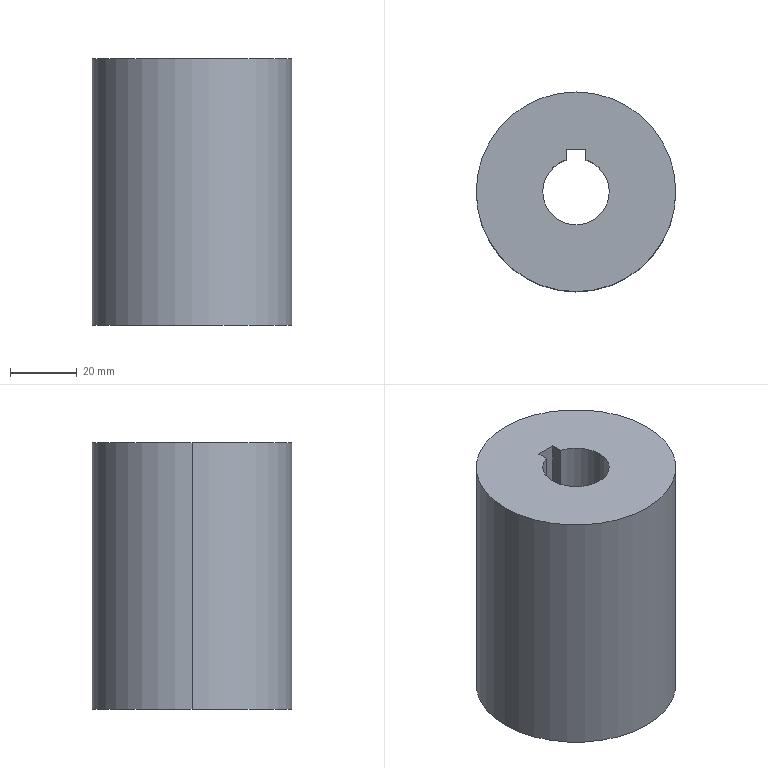Part | SolidWorks | features ICE 4, Extrusion 1 | 1 solid | 15 faces | box 60 x 60 x 80 mm | volume 183532 mm3 | plane 9 | cylinder 6 | commonest cylinder face diameters 20 x3 60 x2 30 x1
STEP:
#1=CARTESIAN_POINT('',(30.,0.,40.));
#2=VERTEX_POINT('',#1);
#3=CARTESIAN_POINT('',(-30.,0.,40.));
#4=VERTEX_POINT('',#3);
#5=CARTESIAN_POINT('',(0.,0.,40.));
#6=DIRECTION('',(0.,0.,1.));
#7=DIRECTION('',(1.,0.,0.));
#8=AXIS2_PLACEMENT_3D('',#5,#6,#7);
#9=CIRCLE('',#8,30.);
#10=EDGE_CURVE('',#2,#4,#9,.T.);
#11=ORIENTED_EDGE('',*,*,#10,.F.);
#12=CARTESIAN_POINT('',(30.,0.,-40.));
#13=VERTEX_POINT('',#12);
#14=CARTESIAN_POINT('',(30.,0.,40.));
#15=DIRECTION('',(0.,0.,-1.));
#16=VECTOR('',#15,1000.);
#17=LINE('',#14,#16);
#18=EDGE_CURVE('',#2,#13,#17,.T.);
#19=ORIENTED_EDGE('',*,*,#18,.T.);
#20=CARTESIAN_POINT('',(-30.,0.,-40.));
#21=VERTEX_POINT('',#20);
#22=CARTESIAN_POINT('',(0.,0.,-40.));
#23=DIRECTION('',(0.,0.,1.));
#24=DIRECTION('',(1.,0.,0.));
#25=AXIS2_PLACEMENT_3D('',#22,#23,#24);
#26=CIRCLE('',#25,30.);
#27=EDGE_CURVE('',#13,#21,#26,.T.);
#28=ORIENTED_EDGE('',*,*,#27,.T.);
#29=CARTESIAN_POINT('',(-30.,0.,40.));
#30=DIRECTION('',(0.,0.,-1.));
#31=VECTOR('',#30,1000.);
#32=LINE('',#29,#31);
#33=EDGE_CURVE('',#4,#21,#32,.T.);
#34=ORIENTED_EDGE('',*,*,#33,.F.);
#35=EDGE_LOOP('',(#11,#19,#28,#34));
#36=FACE_OUTER_BOUND('',#35,.T.);
#37=CARTESIAN_POINT('',(0.,0.,40.));
#38=DIRECTION('',(0.,0.,-1.));
#39=DIRECTION('',(-1.,0.,0.));
#40=AXIS2_PLACEMENT_3D('',#37,#38,#39);
#41=CYLINDRICAL_SURFACE('',#40,30.);
#42=ADVANCED_FACE('',(#36),#41,.T.);
#43=CARTESIAN_POINT('',(-10.,0.,0.));
#44=VERTEX_POINT('',#43);
#45=CARTESIAN_POINT('',(10.,0.,0.));
#46=VERTEX_POINT('',#45);
#47=CARTESIAN_POINT('',(0.,0.,0.));
#48=DIRECTION('',(0.,0.,1.));
#49=DIRECTION('',(-1.,0.,0.));
#50=AXIS2_PLACEMENT_3D('',#47,#48,#49);
#51=CIRCLE('',#50,10.);
#52=EDGE_CURVE('',#44,#46,#51,.T.);
#53=ORIENTED_EDGE('',*,*,#52,.F.);
#54=CARTESIAN_POINT('',(-10.,0.,40.));
#55=VERTEX_POINT('',#54);
#56=CARTESIAN_POINT('',(-10.,0.,-40.));
#57=DIRECTION('',(0.,0.,1.));
#58=VECTOR('',#57,1000.);
#59=LINE('',#56,#58);
#60=EDGE_CURVE('',#44,#55,#59,.T.);
#61=ORIENTED_EDGE('',*,*,#60,.T.);
#62=CARTESIAN_POINT('',(10.,0.,40.));
#63=VERTEX_POINT('',#62);
#64=CARTESIAN_POINT('',(0.,0.,40.));
#65=DIRECTION('',(0.,0.,1.));
#66=DIRECTION('',(1.,0.,0.));
#67=AXIS2_PLACEMENT_3D('',#64,#65,#66);
#68=CIRCLE('',#67,10.);
#69=EDGE_CURVE('',#55,#63,#68,.T.);
#70=ORIENTED_EDGE('',*,*,#69,.T.);
#71=CARTESIAN_POINT('',(10.,0.,-40.));
#72=DIRECTION('',(0.,0.,1.));
#73=VECTOR('',#72,1000.);
#74=LINE('',#71,#73);
#75=EDGE_CURVE('',#46,#63,#74,.T.);
#76=ORIENTED_EDGE('',*,*,#75,.F.);
#77=EDGE_LOOP('',(#53,#61,#70,#76));
#78=FACE_OUTER_BOUND('',#77,.T.);
#79=CARTESIAN_POINT('',(0.,0.,-40.));
#80=DIRECTION('',(0.,0.,1.));
#81=DIRECTION('',(1.,0.,0.));
#82=AXIS2_PLACEMENT_3D('',#79,#80,#81);
#83=CYLINDRICAL_SURFACE('',#82,10.);
#84=ADVANCED_FACE('',(#78),#83,.F.);
#85=CARTESIAN_POINT('',(3.,9.539,0.));
#86=VERTEX_POINT('',#85);
#87=CARTESIAN_POINT('',(0.,0.,0.));
#88=DIRECTION('',(0.,0.,1.));
#89=DIRECTION('',(-1.,0.,0.));
#90=AXIS2_PLACEMENT_3D('',#87,#88,#89);
#91=CIRCLE('',#90,10.);
#92=EDGE_CURVE('',#46,#86,#91,.T.);
#93=ORIENTED_EDGE('',*,*,#92,.F.);
#94=ORIENTED_EDGE('',*,*,#75,.T.);
#95=CARTESIAN_POINT('',(3.,9.539,40.));
#96=VERTEX_POINT('',#95);
#97=CARTESIAN_POINT('',(0.,0.,40.));
#98=DIRECTION('',(0.,0.,1.));
#99=DIRECTION('',(1.,0.,0.));
#100=AXIS2_PLACEMENT_3D('',#97,#98,#99);
#101=CIRCLE('',#100,10.);
#102=EDGE_CURVE('',#63,#96,#101,.T.);
#103=ORIENTED_EDGE('',*,*,#102,.T.);
#104=CARTESIAN_POINT('',(3.,9.539,-40.));
#105=DIRECTION('',(0.,0.,-1.));
#106=VECTOR('',#105,1000.);
#107=LINE('',#104,#106);
#108=EDGE_CURVE('',#96,#86,#107,.T.);
#109=ORIENTED_EDGE('',*,*,#108,.T.);
#110=EDGE_LOOP('',(#93,#94,#103,#109));
#111=FACE_OUTER_BOUND('',#110,.T.);
#112=CARTESIAN_POINT('',(0.,0.,-40.));
#113=DIRECTION('',(0.,0.,1.));
#114=DIRECTION('',(1.,0.,0.));
#115=AXIS2_PLACEMENT_3D('',#112,#113,#114);
#116=CYLINDRICAL_SURFACE('',#115,10.);
#117=ADVANCED_FACE('',(#111),#116,.F.);
#118=ORIENTED_EDGE('',*,*,#60,.F.);
#119=CARTESIAN_POINT('',(-3.,9.539,0.));
#120=VERTEX_POINT('',#119);
#121=CARTESIAN_POINT('',(0.,0.,0.));
#122=DIRECTION('',(0.,0.,1.));
#123=DIRECTION('',(-1.,0.,0.));
#124=AXIS2_PLACEMENT_3D('',#121,#122,#123);
#125=CIRCLE('',#124,10.);
#126=EDGE_CURVE('',#120,#44,#125,.T.);
#127=ORIENTED_EDGE('',*,*,#126,.F.);
#128=CARTESIAN_POINT('',(-3.,9.539,40.));
#129=VERTEX_POINT('',#128);
#130=CARTESIAN_POINT('',(-3.,9.539,-40.));
#131=DIRECTION('',(0.,0.,1.));
#132=VECTOR('',#131,1000.);
#133=LINE('',#130,#132);
#134=EDGE_CURVE('',#120,#129,#133,.T.);
#135=ORIENTED_EDGE('',*,*,#134,.T.);
#136=CARTESIAN_POINT('',(0.,0.,40.));
#137=DIRECTION('',(0.,0.,1.));
#138=DIRECTION('',(1.,0.,0.));
#139=AXIS2_PLACEMENT_3D('',#136,#137,#138);
#140=CIRCLE('',#139,10.);
#141=EDGE_CURVE('',#129,#55,#140,.T.);
#142=ORIENTED_EDGE('',*,*,#141,.T.);
#143=EDGE_LOOP('',(#118,#127,#135,#142));
#144=FACE_OUTER_BOUND('',#143,.T.);
#145=CARTESIAN_POINT('',(0.,0.,-40.));
#146=DIRECTION('',(0.,0.,1.));
#147=DIRECTION('',(1.,0.,0.));
#148=AXIS2_PLACEMENT_3D('',#145,#146,#147);
#149=CYLINDRICAL_SURFACE('',#148,10.);
#150=ADVANCED_FACE('',(#144),#149,.F.);
#151=ORIENTED_EDGE('',*,*,#18,.F.);
#152=CARTESIAN_POINT('',(0.,0.,40.));
#153=DIRECTION('',(0.,0.,1.));
#154=DIRECTION('',(1.,0.,0.));
#155=AXIS2_PLACEMENT_3D('',#152,#153,#154);
#156=CIRCLE('',#155,30.);
#157=EDGE_CURVE('',#4,#2,#156,.T.);
#158=ORIENTED_EDGE('',*,*,#157,.F.);
#159=ORIENTED_EDGE('',*,*,#33,.T.);
#160=CARTESIAN_POINT('',(0.,0.,-40.));
#161=DIRECTION('',(0.,0.,1.));
#162=DIRECTION('',(1.,0.,0.));
#163=AXIS2_PLACEMENT_3D('',#160,#161,#162);
#164=CIRCLE('',#163,30.);
#165=EDGE_CURVE('',#21,#13,#164,.T.);
#166=ORIENTED_EDGE('',*,*,#165,.T.);
#167=EDGE_LOOP('',(#151,#158,#159,#166));
#168=FACE_OUTER_BOUND('',#167,.T.);
#169=CARTESIAN_POINT('',(0.,0.,40.));
#170=DIRECTION('',(0.,0.,-1.));
#171=DIRECTION('',(-1.,0.,0.));
#172=AXIS2_PLACEMENT_3D('',#169,#170,#171);
#173=CYLINDRICAL_SURFACE('',#172,30.);
#174=ADVANCED_FACE('',(#168),#173,.T.);
#175=CARTESIAN_POINT('',(-3.,12.8,40.));
#176=VERTEX_POINT('',#175);
#177=CARTESIAN_POINT('',(-3.,6.87,40.));
#178=DIRECTION('',(0.,-1.,0.));
#179=VECTOR('',#178,1000.);
#180=LINE('',#177,#179);
#181=EDGE_CURVE('',#176,#129,#180,.T.);
#182=ORIENTED_EDGE('',*,*,#181,.F.);
#183=CARTESIAN_POINT('',(3.,12.8,40.));
#184=VERTEX_POINT('',#183);
#185=CARTESIAN_POINT('',(3.,12.8,40.));
#186=DIRECTION('',(-1.,0.,0.));
#187=VECTOR('',#186,1000.);
#188=LINE('',#185,#187);
#189=EDGE_CURVE('',#184,#176,#188,.T.);
#190=ORIENTED_EDGE('',*,*,#189,.F.);
#191=CARTESIAN_POINT('',(3.,6.87,40.));
#192=DIRECTION('',(0.,1.,0.));
#193=VECTOR('',#192,1000.);
#194=LINE('',#191,#193);
#195=EDGE_CURVE('',#96,#184,#194,.T.);
#196=ORIENTED_EDGE('',*,*,#195,.F.);
#197=ORIENTED_EDGE('',*,*,#102,.F.);
#198=ORIENTED_EDGE('',*,*,#69,.F.);
#199=ORIENTED_EDGE('',*,*,#141,.F.);
#200=EDGE_LOOP('',(#182,#190,#196,#197,#198,#199));
#201=FACE_BOUND('',#200,.T.);
#202=ORIENTED_EDGE('',*,*,#157,.T.);
#203=ORIENTED_EDGE('',*,*,#10,.T.);
#204=EDGE_LOOP('',(#202,#203));
#205=FACE_OUTER_BOUND('',#204,.T.);
#206=CARTESIAN_POINT('',(0.,0.,40.));
#207=DIRECTION('',(0.,0.,1.));
#208=DIRECTION('',(1.,0.,0.));
#209=AXIS2_PLACEMENT_3D('',#206,#207,#208);
#210=PLANE('',#209);
#211=ADVANCED_FACE('',(#201,#205),#210,.T.);
#212=CARTESIAN_POINT('',(-14.457,4.,-40.));
#213=VERTEX_POINT('',#212);
#214=CARTESIAN_POINT('',(-14.457,-4.,-40.));
#215=VERTEX_POINT('',#214);
#216=CARTESIAN_POINT('',(0.,0.,-40.));
#217=DIRECTION('',(0.,0.,-1.));
#218=DIRECTION('',(-1.,0.,0.));
#219=AXIS2_PLACEMENT_3D('',#216,#217,#218);
#220=CIRCLE('',#219,15.);
#221=EDGE_CURVE('',#213,#215,#220,.T.);
#222=ORIENTED_EDGE('',*,*,#221,.F.);
#223=CARTESIAN_POINT('',(-18.3,4.,-40.));
#224=VERTEX_POINT('',#223);
#225=CARTESIAN_POINT('',(-18.3,4.,-40.));
#226=DIRECTION('',(1.,0.,0.));
#227=VECTOR('',#226,1000.);
#228=LINE('',#225,#227);
#229=EDGE_CURVE('',#224,#213,#228,.T.);
#230=ORIENTED_EDGE('',*,*,#229,.F.);
#231=CARTESIAN_POINT('',(-18.3,-4.,-40.));
#232=VERTEX_POINT('',#231);
#233=CARTESIAN_POINT('',(-18.3,-4.,-40.));
#234=DIRECTION('',(0.,1.,0.));
#235=VECTOR('',#234,1000.);
#236=LINE('',#233,#235);
#237=EDGE_CURVE('',#232,#224,#236,.T.);
#238=ORIENTED_EDGE('',*,*,#237,.F.);
#239=CARTESIAN_POINT('',(-18.3,-4.,-40.));
#240=DIRECTION('',(-1.,0.,0.));
#241=VECTOR('',#240,1000.);
#242=LINE('',#239,#241);
#243=EDGE_CURVE('',#215,#232,#242,.T.);
#244=ORIENTED_EDGE('',*,*,#243,.F.);
#245=EDGE_LOOP('',(#222,#230,#238,#244));
#246=FACE_BOUND('',#245,.T.);
#247=ORIENTED_EDGE('',*,*,#165,.F.);
#248=ORIENTED_EDGE('',*,*,#27,.F.);
#249=EDGE_LOOP('',(#247,#248));
#250=FACE_OUTER_BOUND('',#249,.T.);
#251=CARTESIAN_POINT('',(0.,0.,-40.));
#252=DIRECTION('',(0.,0.,1.));
#253=DIRECTION('',(1.,0.,0.));
#254=AXIS2_PLACEMENT_3D('',#251,#252,#253);
#255=PLANE('',#254);
#256=ADVANCED_FACE('',(#246,#250),#255,.F.);
#257=CARTESIAN_POINT('',(-18.3,4.,0.));
#258=VERTEX_POINT('',#257);
#259=CARTESIAN_POINT('',(-14.457,4.,0.));
#260=VERTEX_POINT('',#259);
#261=CARTESIAN_POINT('',(-18.3,4.,0.));
#262=DIRECTION('',(1.,0.,0.));
#263=VECTOR('',#262,1000.);
#264=LINE('',#261,#263);
#265=EDGE_CURVE('',#258,#260,#264,.T.);
#266=ORIENTED_EDGE('',*,*,#265,.T.);
#267=CARTESIAN_POINT('',(-14.457,-4.,0.));
#268=VERTEX_POINT('',#267);
#269=CARTESIAN_POINT('',(0.,0.,0.));
#270=DIRECTION('',(0.,0.,-1.));
#271=DIRECTION('',(-1.,0.,0.));
#272=AXIS2_PLACEMENT_3D('',#269,#270,#271);
#273=CIRCLE('',#272,15.);
#274=EDGE_CURVE('',#260,#268,#273,.T.);
#275=ORIENTED_EDGE('',*,*,#274,.T.);
#276=CARTESIAN_POINT('',(-18.3,-4.,0.));
#277=VERTEX_POINT('',#276);
#278=CARTESIAN_POINT('',(-18.3,-4.,0.));
#279=DIRECTION('',(-1.,0.,0.));
#280=VECTOR('',#279,1000.);
#281=LINE('',#278,#280);
#282=EDGE_CURVE('',#268,#277,#281,.T.);
#283=ORIENTED_EDGE('',*,*,#282,.T.);
#284=CARTESIAN_POINT('',(-18.3,-4.,0.));
#285=DIRECTION('',(0.,1.,0.));
#286=VECTOR('',#285,1000.);
#287=LINE('',#284,#286);
#288=EDGE_CURVE('',#277,#258,#287,.T.);
#289=ORIENTED_EDGE('',*,*,#288,.T.);
#290=EDGE_LOOP('',(#266,#275,#283,#289));
#291=FACE_OUTER_BOUND('',#290,.T.);
#292=CARTESIAN_POINT('',(-3.,12.8,0.));
#293=VERTEX_POINT('',#292);
#294=CARTESIAN_POINT('',(-3.,6.87,0.));
#295=DIRECTION('',(0.,-1.,0.));
#296=VECTOR('',#295,1000.);
#297=LINE('',#294,#296);
#298=EDGE_CURVE('',#293,#120,#297,.T.);
#299=ORIENTED_EDGE('',*,*,#298,.T.);
#300=ORIENTED_EDGE('',*,*,#126,.T.);
#301=ORIENTED_EDGE('',*,*,#52,.T.);
#302=ORIENTED_EDGE('',*,*,#92,.T.);
#303=CARTESIAN_POINT('',(3.,12.8,0.));
#304=VERTEX_POINT('',#303);
#305=CARTESIAN_POINT('',(3.,0.,0.));
#306=DIRECTION('',(0.,-1.,0.));
#307=VECTOR('',#306,1000.);
#308=LINE('',#305,#307);
#309=EDGE_CURVE('',#304,#86,#308,.T.);
#310=ORIENTED_EDGE('',*,*,#309,.F.);
#311=CARTESIAN_POINT('',(3.,12.8,0.));
#312=DIRECTION('',(-1.,0.,0.));
#313=VECTOR('',#312,1000.);
#314=LINE('',#311,#313);
#315=EDGE_CURVE('',#304,#293,#314,.T.);
#316=ORIENTED_EDGE('',*,*,#315,.T.);
#317=EDGE_LOOP('',(#299,#300,#301,#302,#310,#316));
#318=FACE_BOUND('',#317,.T.);
#319=CARTESIAN_POINT('',(0.,0.,0.));
#320=DIRECTION('',(0.,0.,-1.));
#321=DIRECTION('',(-1.,0.,0.));
#322=AXIS2_PLACEMENT_3D('',#319,#320,#321);
#323=PLANE('',#322);
#324=ADVANCED_FACE('',(#291,#318),#323,.T.);
#325=ORIENTED_EDGE('',*,*,#274,.F.);
#326=CARTESIAN_POINT('',(-14.457,4.,0.));
#327=DIRECTION('',(0.,0.,-1.));
#328=VECTOR('',#327,1000.);
#329=LINE('',#326,#328);
#330=EDGE_CURVE('',#260,#213,#329,.T.);
#331=ORIENTED_EDGE('',*,*,#330,.T.);
#332=ORIENTED_EDGE('',*,*,#221,.T.);
#333=CARTESIAN_POINT('',(-14.457,-4.,0.));
#334=DIRECTION('',(0.,0.,1.));
#335=VECTOR('',#334,1000.);
#336=LINE('',#333,#335);
#337=EDGE_CURVE('',#215,#268,#336,.T.);
#338=ORIENTED_EDGE('',*,*,#337,.T.);
#339=EDGE_LOOP('',(#325,#331,#332,#338));
#340=FACE_OUTER_BOUND('',#339,.T.);
#341=CARTESIAN_POINT('',(0.,0.,0.));
#342=DIRECTION('',(0.,0.,-1.));
#343=DIRECTION('',(-1.,0.,0.));
#344=AXIS2_PLACEMENT_3D('',#341,#342,#343);
#345=CYLINDRICAL_SURFACE('',#344,15.);
#346=ADVANCED_FACE('',(#340),#345,.F.);
#347=ORIENTED_EDGE('',*,*,#298,.F.);
#348=CARTESIAN_POINT('',(-3.,12.8,0.));
#349=DIRECTION('',(0.,0.,1.));
#350=VECTOR('',#349,1000.);
#351=LINE('',#348,#350);
#352=EDGE_CURVE('',#293,#176,#351,.T.);
#353=ORIENTED_EDGE('',*,*,#352,.T.);
#354=ORIENTED_EDGE('',*,*,#181,.T.);
#355=ORIENTED_EDGE('',*,*,#134,.F.);
#356=EDGE_LOOP('',(#347,#353,#354,#355));
#357=FACE_OUTER_BOUND('',#356,.T.);
#358=CARTESIAN_POINT('',(-3.,6.87,0.));
#359=DIRECTION('',(-1.,0.,0.));
#360=DIRECTION('',(0.,-1.,0.));
#361=AXIS2_PLACEMENT_3D('',#358,#359,#360);
#362=PLANE('',#361);
#363=ADVANCED_FACE('',(#357),#362,.F.);
#364=ORIENTED_EDGE('',*,*,#195,.T.);
#365=CARTESIAN_POINT('',(3.,12.8,0.));
#366=DIRECTION('',(0.,0.,1.));
#367=VECTOR('',#366,1000.);
#368=LINE('',#365,#367);
#369=EDGE_CURVE('',#304,#184,#368,.T.);
#370=ORIENTED_EDGE('',*,*,#369,.F.);
#371=ORIENTED_EDGE('',*,*,#309,.T.);
#372=ORIENTED_EDGE('',*,*,#108,.F.);
#373=EDGE_LOOP('',(#364,#370,#371,#372));
#374=FACE_OUTER_BOUND('',#373,.T.);
#375=CARTESIAN_POINT('',(3.,6.87,0.));
#376=DIRECTION('',(1.,0.,0.));
#377=DIRECTION('',(0.,1.,0.));
#378=AXIS2_PLACEMENT_3D('',#375,#376,#377);
#379=PLANE('',#378);
#380=ADVANCED_FACE('',(#374),#379,.F.);
#381=ORIENTED_EDGE('',*,*,#189,.T.);
#382=ORIENTED_EDGE('',*,*,#352,.F.);
#383=ORIENTED_EDGE('',*,*,#315,.F.);
#384=ORIENTED_EDGE('',*,*,#369,.T.);
#385=EDGE_LOOP('',(#381,#382,#383,#384));
#386=FACE_OUTER_BOUND('',#385,.T.);
#387=CARTESIAN_POINT('',(3.,12.8,0.));
#388=DIRECTION('',(0.,1.,0.));
#389=DIRECTION('',(-1.,0.,0.));
#390=AXIS2_PLACEMENT_3D('',#387,#388,#389);
#391=PLANE('',#390);
#392=ADVANCED_FACE('',(#386),#391,.F.);
#393=ORIENTED_EDGE('',*,*,#265,.F.);
#394=CARTESIAN_POINT('',(-18.3,4.,0.));
#395=DIRECTION('',(0.,0.,-1.));
#396=VECTOR('',#395,1000.);
#397=LINE('',#394,#396);
#398=EDGE_CURVE('',#258,#224,#397,.T.);
#399=ORIENTED_EDGE('',*,*,#398,.T.);
#400=ORIENTED_EDGE('',*,*,#229,.T.);
#401=ORIENTED_EDGE('',*,*,#330,.F.);
#402=EDGE_LOOP('',(#393,#399,#400,#401));
#403=FACE_OUTER_BOUND('',#402,.T.);
#404=CARTESIAN_POINT('',(-18.3,4.,0.));
#405=DIRECTION('',(0.,1.,0.));
#406=DIRECTION('',(0.,0.,1.));
#407=AXIS2_PLACEMENT_3D('',#404,#405,#406);
#408=PLANE('',#407);
#409=ADVANCED_FACE('',(#403),#408,.F.);
#410=ORIENTED_EDGE('',*,*,#243,.T.);
#411=CARTESIAN_POINT('',(-18.3,-4.,0.));
#412=DIRECTION('',(0.,0.,-1.));
#413=VECTOR('',#412,1000.);
#414=LINE('',#411,#413);
#415=EDGE_CURVE('',#277,#232,#414,.T.);
#416=ORIENTED_EDGE('',*,*,#415,.F.);
#417=ORIENTED_EDGE('',*,*,#282,.F.);
#418=ORIENTED_EDGE('',*,*,#337,.F.);
#419=EDGE_LOOP('',(#410,#416,#417,#418));
#420=FACE_OUTER_BOUND('',#419,.T.);
#421=CARTESIAN_POINT('',(-18.3,-4.,0.));
#422=DIRECTION('',(0.,-1.,0.));
#423=DIRECTION('',(0.,0.,-1.));
#424=AXIS2_PLACEMENT_3D('',#421,#422,#423);
#425=PLANE('',#424);
#426=ADVANCED_FACE('',(#420),#425,.F.);
#427=ORIENTED_EDGE('',*,*,#237,.T.);
#428=ORIENTED_EDGE('',*,*,#398,.F.);
#429=ORIENTED_EDGE('',*,*,#288,.F.);
#430=ORIENTED_EDGE('',*,*,#415,.T.);
#431=EDGE_LOOP('',(#427,#428,#429,#430));
#432=FACE_OUTER_BOUND('',#431,.T.);
#433=CARTESIAN_POINT('',(-18.3,-4.,0.));
#434=DIRECTION('',(-1.,0.,0.));
#435=DIRECTION('',(0.,-1.,0.));
#436=AXIS2_PLACEMENT_3D('',#433,#434,#435);
#437=PLANE('',#436);
#438=ADVANCED_FACE('',(#432),#437,.F.);
#439=CLOSED_SHELL('',(#42,#84,#117,#150,#174,#211,#256,#324,#346,#363,#380,#392,#409,#426,#438));
#440=MANIFOLD_SOLID_BREP('',#439);
#441=CARTESIAN_POINT('',(0.,0.,0.));
#442=DIRECTION('',(0.,0.,1.));
#443=DIRECTION('',(1.,0.,0.));
#444=AXIS2_PLACEMENT_3D('',#441,#442,#443);
#445=(LENGTH_UNIT()NAMED_UNIT(*)SI_UNIT(.MILLI.,.METRE.));
#446=UNCERTAINTY_MEASURE_WITH_UNIT(LENGTH_MEASURE(0.00001),#445,'','');
#447=(NAMED_UNIT(*)PLANE_ANGLE_UNIT()SI_UNIT($,.RADIAN.));
#448=(NAMED_UNIT(*)SI_UNIT($,.STERADIAN.)SOLID_ANGLE_UNIT());
#449=(GEOMETRIC_REPRESENTATION_CONTEXT(3)GLOBAL_UNCERTAINTY_ASSIGNED_CONTEXT((#446))GLOBAL_UNIT_ASSIGNED_CONTEXT((#445,#447,#448))REPRESENTATION_CONTEXT('',''));
#450=ADVANCED_BREP_SHAPE_REPRESENTATION('',(#440,#444),#449);